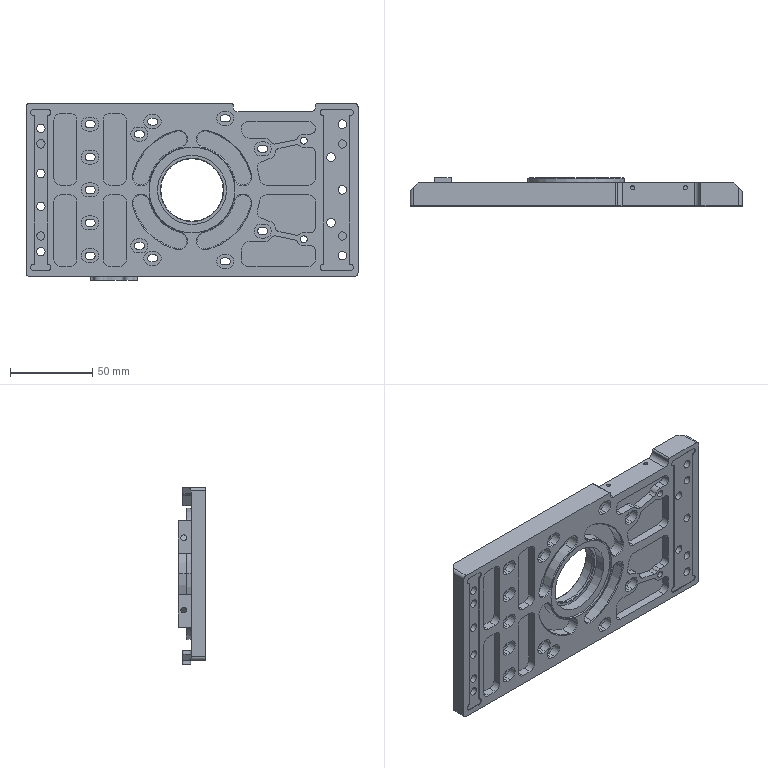NC program | Mastercam | posted with a generic post | part box 202 x 17 x 107.5 mm
Lines 9004 to 9381 of 36425:
(10 FEM |TOOL - 11|DIA. OFF. - 11|LEN. - 11|TOOL DIA. - 10.)
N8170 T11 M6
N8172 G0 G54 G90 X105.364 Y-56.157 C0. B0. S6000 M3
N8174 G43 H11 Z100.
N8176 Z1.
N8178 G1 Z-16.8 F600.
N8180 X104.657 Y-55.45 F1000.
N8182 G3 X104.303 Y-55.303 I-.354 J-.353
N8184 X103.95 Y-55.45 J-.5
N8186 G2 X99. Y-57.5 I-4.95 J4.95
N8188 G1 X-99.
N8190 G2 X-106. Y-50.5 J7.
N8192 G1 Y50.5
N8194 G2 X-99. Y57.5 I7.
N8196 G1 X24.
N8198 G2 X29.916 Y52.5 J-6.
N8200 G1 X70.084
N8202 G2 X76. Y57.5 I5.916 J-1.
N8204 G1 X99.
N8206 G2 X106. Y50.5 J-7.
N8208 G1 Y-50.5
N8210 G2 X103.584 Y-55.79 I-7.
N8212 G3 X103.411 Y-56.168 I.327 J-.378
N8214 X103.533 Y-56.496 I.5
N8216 G1 X104.188 Y-57.251
N8218 Z-15.8 F1200.
N8220 G0 Z100.
N8222 X-12.51 Y.5
N8224 Z-9.5
N8226 G1 Z-10.5 F600.
N8228 X-13.51 F1000.
N8230 G3 X-14.01 Y0. J-.5
N8232 X0. Y-14.01 I14.01
N8234 X14.01 Y0. J14.01
N8236 X0. Y14.01 I-14.01
N8238 X-14.01 Y0. J-14.01
N8240 X-14.001 Y-.5 I14.01
N8242 X-13.501 Y-.982 I.5 J.018
N8244 G1 X-13.484
N8246 X-12.484 Y-.946
N8248 Z-9.5 F1200.
N8250 G0 Z100.
(TO)
N8252 X-14.47 Y.5
N8254 Z-6.8
N8256 G1 Z-7.8 F600.
N8258 G41 D11 X-15.47 F1000.
N8260 G3 X-15.97 Y0. J-.5
N8262 X0. Y-15.97 I15.97
N8264 X15.97 Y0. J15.97
N8266 X0. Y15.97 I-15.97
N8268 X-15.97 Y0. J-15.97
N8270 X-15.962 Y-.5 I15.97
N8272 X-15.462 Y-.984 I.5 J.016
N8274 G1 X-15.447
N8276 G40 X-14.447 Y-.953
N8278 Z-6.8 F1200.
N8280 G0 Z100.
N8282 X-19.6 Y.5
N8284 Z-.5
N8286 G1 Z-1.5 F600.
N8288 X-20.6 F1000.
N8290 G3 X-21.1 Y0. J-.5
N8292 X0. Y-21.1 I21.1
N8294 X21.1 Y0. J21.1
N8296 X0. Y21.1 I-21.1
N8298 X-21.1 Y0. J-21.1
N8300 X-21.094 Y-.5 I21.1
N8302 X-20.594 Y-.988 I.5 J.012
N8304 G1 X-20.582
N8306 X-19.583 Y-.964
N8308 Z-.5 F1200.
N8310 G0 Z100.
N8312 M5
N8314 G0 G28 G91 Z0.
N8316 G28
N8318 M01
N8320 G0 G17 G40 G80 G90 G94 G98
N8322 G0 G28 G91 Z0.
(8 FEM |TOOL - 8|DIA. OFF. - 8|LEN. - 8|TOOL DIA. - 8.)
N8324 T8 M6
N8326 G0 G54 G90 X-44.1 Y42.4 C0. B0. S10000 M3
N8328 G43 H8 Z100.
N8330 Z1.
N8332 G1 Z0. F600.
N8334 X-49.9 Z-.035 F4000.
N8336 Y7.1 Z-.25
N8338 X-44.1 Z-.285
N8340 Y42.4 Z-.5
N8342 X-49.9 Z-.535
N8344 Y7.1 Z-.75
N8346 X-44.1 Z-.785
N8348 Y42.4 Z-1.
N8350 X-49.9 Z-1.035
N8352 Y7.1 Z-1.25
N8354 X-44.1 Z-1.285
N8356 Y42.4 Z-1.5
N8358 X-49.9 Z-1.535
N8360 Y7.1 Z-1.75
N8362 X-44.1 Z-1.785
N8364 Y42.4 Z-2.
N8366 X-49.9 Z-2.035
N8368 Y7.1 Z-2.25
N8370 X-44.1 Z-2.285
N8372 Y42.4 Z-2.5
N8374 X-49.9 Z-2.535
N8376 Y7.1 Z-2.75
N8378 X-44.1 Z-2.785
N8380 Y42.4 Z-3.
N8382 X-49.9 Z-3.035
N8384 Y7.1 Z-3.25
N8386 X-44.1 Z-3.285
N8388 Y42.4 Z-3.5
N8390 X-49.9 Z-3.535
N8392 Y7.1 Z-3.75
N8394 X-44.1 Z-3.785
N8396 Y42.4 Z-4.
N8398 X-49.9 Z-4.035
N8400 Y7.1 Z-4.25
N8402 X-44.1 Z-4.285
N8404 Y42.4 Z-4.5
N8406 X-49.9 Z-4.535
N8408 Y7.1 Z-4.75
N8410 X-44.1 Z-4.785
N8412 Y25.96 Z-4.9
N8414 Y42.4
N8416 X-49.9
N8418 Y7.1
N8420 X-44.1
N8422 Y26.46
N8424 Z-3.9 F1200.
N8426 G0 Z100.
N8428 X-74.1 Y42.4
N8430 Z1.
N8432 G1 Z0. F600.
N8434 X-79.9 Z-.035 F4000.
N8436 Y7.1 Z-.25
N8438 X-74.1 Z-.285
N8440 Y42.4 Z-.5
N8442 X-79.9 Z-.535
N8444 Y7.1 Z-.75
N8446 X-74.1 Z-.785
N8448 Y42.4 Z-1.
N8450 X-79.9 Z-1.035
N8452 Y7.1 Z-1.25
N8454 X-74.1 Z-1.285
N8456 Y42.4 Z-1.5
N8458 X-79.9 Z-1.535
N8460 Y7.1 Z-1.75
N8462 X-74.1 Z-1.785
N8464 Y42.4 Z-2.
N8466 X-79.9 Z-2.035
N8468 Y7.1 Z-2.25
N8470 X-74.1 Z-2.285
N8472 Y42.4 Z-2.5
N8474 X-79.9 Z-2.535
N8476 Y7.1 Z-2.75
N8478 X-74.1 Z-2.785
N8480 Y42.4 Z-3.
N8482 X-79.9 Z-3.035
N8484 Y7.1 Z-3.25
N8486 X-74.1 Z-3.285
N8488 Y42.4 Z-3.5
N8490 X-79.9 Z-3.535
N8492 Y7.1 Z-3.75
N8494 X-74.1 Z-3.785
N8496 Y42.4 Z-4.
N8498 X-79.9 Z-4.035
N8500 Y7.1 Z-4.25
N8502 X-74.1 Z-4.285
N8504 Y42.4 Z-4.5
N8506 X-79.9 Z-4.535
N8508 Y7.1 Z-4.75
N8510 X-74.1 Z-4.785
N8512 Y25.96 Z-4.9
N8514 Y42.4
N8516 X-79.9
N8518 Y7.1
N8520 X-74.1
N8522 Y26.46
N8524 Z-3.9 F1200.
N8526 G0 Z100.
N8528 Y-7.1
N8530 Z1.
N8532 G1 Z0. F600.
N8534 X-79.9 Z-.035 F4000.
N8536 Y-42.4 Z-.25
N8538 X-74.1 Z-.285
N8540 Y-7.1 Z-.5
N8542 X-79.9 Z-.535
N8544 Y-42.4 Z-.75
N8546 X-74.1 Z-.785
N8548 Y-7.1 Z-1.
N8550 X-79.9 Z-1.035
N8552 Y-42.4 Z-1.25
N8554 X-74.1 Z-1.285
N8556 Y-7.1 Z-1.5
N8558 X-79.9 Z-1.535
N8560 Y-42.4 Z-1.75
N8562 X-74.1 Z-1.785
N8564 Y-7.1 Z-2.
N8566 X-79.9 Z-2.035
N8568 Y-42.4 Z-2.25
N8570 X-74.1 Z-2.285
N8572 Y-7.1 Z-2.5
N8574 X-79.9 Z-2.535
N8576 Y-42.4 Z-2.75
N8578 X-74.1 Z-2.785
N8580 Y-7.1 Z-3.
N8582 X-79.9 Z-3.035
N8584 Y-42.4 Z-3.25
N8586 X-74.1 Z-3.285
N8588 Y-7.1 Z-3.5
N8590 X-79.9 Z-3.535
N8592 Y-42.4 Z-3.75
N8594 X-74.1 Z-3.785
N8596 Y-7.1 Z-4.
N8598 X-79.9 Z-4.035
N8600 Y-42.4 Z-4.25
N8602 X-74.1 Z-4.285
N8604 Y-7.1 Z-4.5
N8606 X-79.9 Z-4.535
N8608 Y-42.4 Z-4.75
N8610 X-74.1 Z-4.785
N8612 Y-23.54 Z-4.9
N8614 Y-7.1
N8616 X-79.9
N8618 Y-42.4
N8620 X-74.1
N8622 Y-23.04
N8624 Z-3.9 F1200.
N8626 G0 Z100.
N8628 X-44.1 Y-7.1
N8630 Z1.
N8632 G1 Z0. F600.
N8634 X-49.9 Z-.035 F4000.
N8636 Y-42.4 Z-.25
N8638 X-44.1 Z-.285
N8640 Y-7.1 Z-.5
N8642 X-49.9 Z-.535
N8644 Y-42.4 Z-.75
N8646 X-44.1 Z-.785
N8648 Y-7.1 Z-1.
N8650 X-49.9 Z-1.035
N8652 Y-42.4 Z-1.25
N8654 X-44.1 Z-1.285
N8656 Y-7.1 Z-1.5
N8658 X-49.9 Z-1.535
N8660 Y-42.4 Z-1.75
N8662 X-44.1 Z-1.785
N8664 Y-7.1 Z-2.
N8666 X-49.9 Z-2.035
N8668 Y-42.4 Z-2.25
N8670 X-44.1 Z-2.285
N8672 Y-7.1 Z-2.5
N8674 X-49.9 Z-2.535
N8676 Y-42.4 Z-2.75
N8678 X-44.1 Z-2.785
N8680 Y-7.1 Z-3.
N8682 X-49.9 Z-3.035
N8684 Y-42.4 Z-3.25
N8686 X-44.1 Z-3.285
N8688 Y-7.1 Z-3.5
N8690 X-49.9 Z-3.535
N8692 Y-42.4 Z-3.75
N8694 X-44.1 Z-3.785
N8696 Y-7.1 Z-4.
N8698 X-49.9 Z-4.035
N8700 Y-42.4 Z-4.25
N8702 X-44.1 Z-4.285
N8704 Y-7.1 Z-4.5
N8706 X-49.9 Z-4.535
N8708 Y-42.4 Z-4.75
N8710 X-44.1 Z-4.785
N8712 Y-23.54 Z-4.9
N8714 Y-7.1
N8716 X-49.9
N8718 Y-42.4
N8720 X-44.1
N8722 Y-23.04
N8724 Z-3.9 F1200.
N8726 G0 Z100.
N8728 X-46.6 Y41.31
N8730 Z-4.
N8732 G1 Z-5. F600.
N8734 Y42.11 F1000.
N8736 G3 X-47. Y42.51 I-.4
N8738 G1 X-50.
N8740 G3 X-50.01 Y42.5 J-.01
N8742 G1 Y7.
N8744 G3 X-50. Y6.99 I.01
N8746 G1 X-44.
N8748 G3 X-43.99 Y7. J.01
N8750 G1 Y42.5
N8752 G3 X-44. Y42.51 I-.01
N8754 G1 X-47.
N8756 X-47.5
N8758 G3 X-47.9 Y42.11 J-.4
N8760 G1 Y41.31
N8762 Z-4. F1200.
N8764 G0 Z100.
N8766 X-76.6
N8768 Z-4.
N8770 G1 Z-5. F600.
N8772 Y42.11 F1000.
N8774 G3 X-77. Y42.51 I-.4
N8776 G1 X-80.
N8778 G3 X-80.01 Y42.5 J-.01
N8780 G1 Y7.
N8782 G3 X-80. Y6.99 I.01
N8784 G1 X-74.
N8786 G3 X-73.99 Y7. J.01
N8788 G1 Y42.5
N8790 G3 X-74. Y42.51 I-.01
N8792 G1 X-77.
N8794 X-77.5
N8796 G3 X-77.9 Y42.11 J-.4
N8798 G1 Y41.31
N8800 Z-4. F1200.
N8802 G0 Z100.
N8804 X-76.6 Y-8.19
N8806 Z-4.
N8808 G1 Z-5. F600.
N8810 Y-7.39 F1000.
N8812 G3 X-77. Y-6.99 I-.4
N8814 G1 X-80.
N8816 G3 X-80.01 Y-7. J-.01
N8818 G1 Y-42.5
N8820 G3 X-80. Y-42.51 I.01
N8822 G1 X-74.
N8824 G3 X-73.99 Y-42.5 J.01
N8826 G1 Y-7.
N8828 G3 X-74. Y-6.99 I-.01
N8830 G1 X-77.
N8832 X-77.5
N8834 G3 X-77.9 Y-7.39 J-.4
N8836 G1 Y-8.19
N8838 Z-4. F1200.
N8840 G0 Z100.
N8842 X-46.6
N8844 Z-4.
N8846 G1 Z-5. F600.
N8848 Y-7.39 F1000.
N8850 G3 X-47. Y-6.99 I-.4
N8852 G1 X-50.
N8854 G3 X-50.01 Y-7. J-.01
N8856 G1 Y-42.5
N8858 G3 X-50. Y-42.51 I.01
N8860 G1 X-44.
N8862 G3 X-43.99 Y-42.5 J.01
N8864 G1 Y-7.
N8866 G3 X-44. Y-6.99 I-.01
N8868 G1 X-47.
N8870 X-47.5
N8872 G3 X-47.9 Y-7.39 J-.4
N8874 G1 Y-8.19
N8876 Z-4. F1200.
N8878 G0 Z100.
N8880 X92. Y45.
N8882 Z1.
N8884 G1 Z0. F600.
N8886 X84. Z-.024 F4000.
N8888 Y-45. Z-.3
N8890 X92. Z-.324
N8892 Y-20.333 Z-.4
N8894 Y45.
N8896 X84.
N8898 Y-45.
N8900 X92.
N8902 Y-19.833
N8904 Z.6 F1200.
N8906 G0 Z100.
N8908 M5
N8910 G0 G28 G91 Z0.
N8912 G28
N8914 M01
N8916 G0 G17 G40 G80 G90 G94 G98
N8918 G0 G28 G91 Z0.